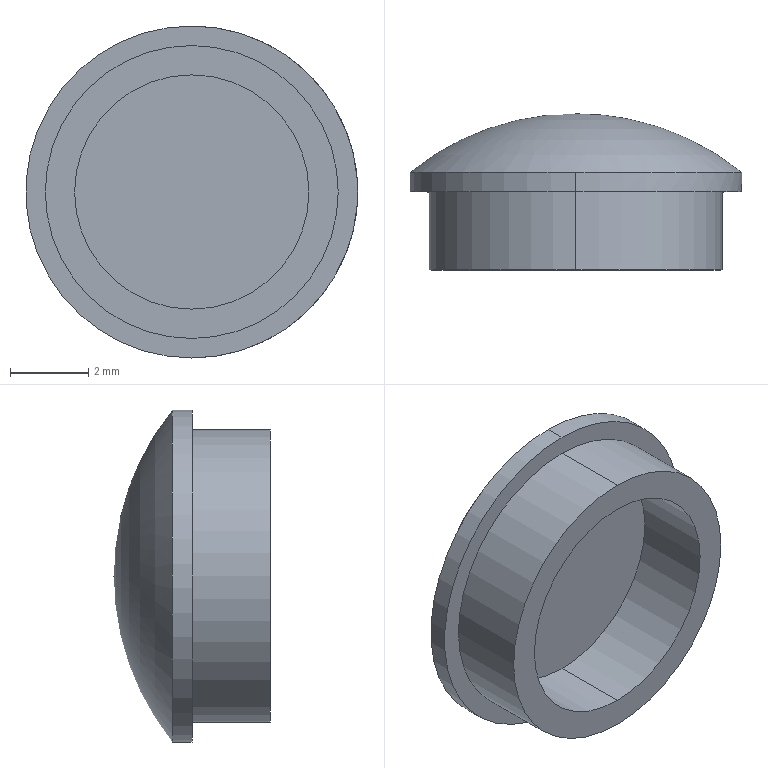Part | SolidWorks | features ICE 2, Dome 1, Extrusion 1, Scale 1 | 1 solid | 10 faces | box 8.5 x 4 x 8.5 mm | volume 104.507 mm3 | cylinder 6 | plane 3 | sphere 1 | commonest cylinder face diameters 6 x2 7.5 x2 8.5 x2
STEP:
#1=CARTESIAN_POINT('',(0.0000104,4.192,3.));
#2=VERTEX_POINT('',#1);
#3=CARTESIAN_POINT('',(0.0000104,4.192,-3.));
#4=VERTEX_POINT('',#3);
#5=CARTESIAN_POINT('',(0.0000104,4.192,0.0001016));
#6=DIRECTION('',(0.,-1.,0.));
#7=DIRECTION('',(0.,0.,-1.));
#8=AXIS2_PLACEMENT_3D('',#5,#6,#7);
#9=CIRCLE('',#8,3.);
#10=EDGE_CURVE('',#2,#4,#9,.T.);
#11=ORIENTED_EDGE('',*,*,#10,.F.);
#12=CARTESIAN_POINT('',(0.0000104,2.192,3.));
#13=VERTEX_POINT('',#12);
#14=CARTESIAN_POINT('',(0.0000104,4.192,3.));
#15=DIRECTION('',(0.,-1.,0.));
#16=VECTOR('',#15,1000.);
#17=LINE('',#14,#16);
#18=EDGE_CURVE('',#2,#13,#17,.T.);
#19=ORIENTED_EDGE('',*,*,#18,.T.);
#20=CARTESIAN_POINT('',(0.0000104,2.192,-3.));
#21=VERTEX_POINT('',#20);
#22=CARTESIAN_POINT('',(0.0000104,2.192,0.0001016));
#23=DIRECTION('',(0.,-1.,0.));
#24=DIRECTION('',(0.,0.,-1.));
#25=AXIS2_PLACEMENT_3D('',#22,#23,#24);
#26=CIRCLE('',#25,3.);
#27=EDGE_CURVE('',#13,#21,#26,.T.);
#28=ORIENTED_EDGE('',*,*,#27,.T.);
#29=CARTESIAN_POINT('',(0.0000104,4.192,-3.));
#30=DIRECTION('',(0.,-1.,0.));
#31=VECTOR('',#30,1000.);
#32=LINE('',#29,#31);
#33=EDGE_CURVE('',#4,#21,#32,.T.);
#34=ORIENTED_EDGE('',*,*,#33,.F.);
#35=EDGE_LOOP('',(#11,#19,#28,#34));
#36=FACE_OUTER_BOUND('',#35,.T.);
#37=CARTESIAN_POINT('',(0.0000104,4.192,0.0001016));
#38=DIRECTION('',(0.,-1.,0.));
#39=DIRECTION('',(0.,0.,-1.));
#40=AXIS2_PLACEMENT_3D('',#37,#38,#39);
#41=CYLINDRICAL_SURFACE('',#40,3.);
#42=ADVANCED_FACE('',(#36),#41,.F.);
#43=CARTESIAN_POINT('',(0.0000104,4.692,4.25));
#44=VERTEX_POINT('',#43);
#45=CARTESIAN_POINT('',(0.0000104,4.692,-4.25));
#46=VERTEX_POINT('',#45);
#47=CARTESIAN_POINT('',(0.0000104,4.692,0.0001016));
#48=DIRECTION('',(0.,1.,0.));
#49=DIRECTION('',(0.,0.,1.));
#50=AXIS2_PLACEMENT_3D('',#47,#48,#49);
#51=CIRCLE('',#50,4.25);
#52=EDGE_CURVE('',#44,#46,#51,.T.);
#53=ORIENTED_EDGE('',*,*,#52,.F.);
#54=CARTESIAN_POINT('',(0.0000104,4.192,4.25));
#55=VERTEX_POINT('',#54);
#56=CARTESIAN_POINT('',(0.0000104,4.692,4.25));
#57=DIRECTION('',(0.,-1.,0.));
#58=VECTOR('',#57,1000.);
#59=LINE('',#56,#58);
#60=EDGE_CURVE('',#44,#55,#59,.T.);
#61=ORIENTED_EDGE('',*,*,#60,.T.);
#62=CARTESIAN_POINT('',(0.0000104,4.192,-4.25));
#63=VERTEX_POINT('',#62);
#64=CARTESIAN_POINT('',(0.0000104,4.192,0.0001016));
#65=DIRECTION('',(0.,1.,0.));
#66=DIRECTION('',(0.,0.,1.));
#67=AXIS2_PLACEMENT_3D('',#64,#65,#66);
#68=CIRCLE('',#67,4.25);
#69=EDGE_CURVE('',#55,#63,#68,.T.);
#70=ORIENTED_EDGE('',*,*,#69,.T.);
#71=CARTESIAN_POINT('',(0.0000104,4.692,-4.25));
#72=DIRECTION('',(0.,-1.,0.));
#73=VECTOR('',#72,1000.);
#74=LINE('',#71,#73);
#75=EDGE_CURVE('',#46,#63,#74,.T.);
#76=ORIENTED_EDGE('',*,*,#75,.F.);
#77=EDGE_LOOP('',(#53,#61,#70,#76));
#78=FACE_OUTER_BOUND('',#77,.T.);
#79=CARTESIAN_POINT('',(0.0000104,4.692,0.0001016));
#80=DIRECTION('',(0.,-1.,0.));
#81=DIRECTION('',(0.,0.,-1.));
#82=AXIS2_PLACEMENT_3D('',#79,#80,#81);
#83=CYLINDRICAL_SURFACE('',#82,4.25);
#84=ADVANCED_FACE('',(#78),#83,.T.);
#85=CARTESIAN_POINT('',(0.0000104,4.192,3.75));
#86=VERTEX_POINT('',#85);
#87=CARTESIAN_POINT('',(0.0000104,4.192,-3.75));
#88=VERTEX_POINT('',#87);
#89=CARTESIAN_POINT('',(0.0000104,4.192,0.0001016));
#90=DIRECTION('',(0.,1.,0.));
#91=DIRECTION('',(0.,0.,1.));
#92=AXIS2_PLACEMENT_3D('',#89,#90,#91);
#93=CIRCLE('',#92,3.75);
#94=EDGE_CURVE('',#86,#88,#93,.T.);
#95=ORIENTED_EDGE('',*,*,#94,.F.);
#96=CARTESIAN_POINT('',(0.0000104,2.192,3.75));
#97=VERTEX_POINT('',#96);
#98=CARTESIAN_POINT('',(0.0000104,4.192,3.75));
#99=DIRECTION('',(0.,-1.,0.));
#100=VECTOR('',#99,1000.);
#101=LINE('',#98,#100);
#102=EDGE_CURVE('',#86,#97,#101,.T.);
#103=ORIENTED_EDGE('',*,*,#102,.T.);
#104=CARTESIAN_POINT('',(0.0000104,2.192,-3.75));
#105=VERTEX_POINT('',#104);
#106=CARTESIAN_POINT('',(0.0000104,2.192,0.0001016));
#107=DIRECTION('',(0.,1.,0.));
#108=DIRECTION('',(0.,0.,1.));
#109=AXIS2_PLACEMENT_3D('',#106,#107,#108);
#110=CIRCLE('',#109,3.75);
#111=EDGE_CURVE('',#97,#105,#110,.T.);
#112=ORIENTED_EDGE('',*,*,#111,.T.);
#113=CARTESIAN_POINT('',(0.0000104,4.192,-3.75));
#114=DIRECTION('',(0.,-1.,0.));
#115=VECTOR('',#114,1000.);
#116=LINE('',#113,#115);
#117=EDGE_CURVE('',#88,#105,#116,.T.);
#118=ORIENTED_EDGE('',*,*,#117,.F.);
#119=EDGE_LOOP('',(#95,#103,#112,#118));
#120=FACE_OUTER_BOUND('',#119,.T.);
#121=CARTESIAN_POINT('',(0.0000104,4.192,0.0001016));
#122=DIRECTION('',(0.,-1.,0.));
#123=DIRECTION('',(0.,0.,-1.));
#124=AXIS2_PLACEMENT_3D('',#121,#122,#123);
#125=CYLINDRICAL_SURFACE('',#124,3.75);
#126=ADVANCED_FACE('',(#120),#125,.T.);
#127=ORIENTED_EDGE('',*,*,#102,.F.);
#128=CARTESIAN_POINT('',(0.0000104,4.192,0.0001016));
#129=DIRECTION('',(0.,1.,0.));
#130=DIRECTION('',(0.,0.,1.));
#131=AXIS2_PLACEMENT_3D('',#128,#129,#130);
#132=CIRCLE('',#131,3.75);
#133=EDGE_CURVE('',#88,#86,#132,.T.);
#134=ORIENTED_EDGE('',*,*,#133,.F.);
#135=ORIENTED_EDGE('',*,*,#117,.T.);
#136=CARTESIAN_POINT('',(0.0000104,2.192,0.0001016));
#137=DIRECTION('',(0.,1.,0.));
#138=DIRECTION('',(0.,0.,1.));
#139=AXIS2_PLACEMENT_3D('',#136,#137,#138);
#140=CIRCLE('',#139,3.75);
#141=EDGE_CURVE('',#105,#97,#140,.T.);
#142=ORIENTED_EDGE('',*,*,#141,.T.);
#143=EDGE_LOOP('',(#127,#134,#135,#142));
#144=FACE_OUTER_BOUND('',#143,.T.);
#145=CARTESIAN_POINT('',(0.0000104,4.192,0.0001016));
#146=DIRECTION('',(0.,-1.,0.));
#147=DIRECTION('',(0.,0.,-1.));
#148=AXIS2_PLACEMENT_3D('',#145,#146,#147);
#149=CYLINDRICAL_SURFACE('',#148,3.75);
#150=ADVANCED_FACE('',(#144),#149,.T.);
#151=CARTESIAN_POINT('',(0.0000104,2.192,0.0001016));
#152=DIRECTION('',(0.,-1.,0.));
#153=DIRECTION('',(0.,0.,-1.));
#154=AXIS2_PLACEMENT_3D('',#151,#152,#153);
#155=CIRCLE('',#154,3.);
#156=EDGE_CURVE('',#21,#13,#155,.T.);
#157=ORIENTED_EDGE('',*,*,#156,.F.);
#158=ORIENTED_EDGE('',*,*,#27,.F.);
#159=EDGE_LOOP('',(#157,#158));
#160=FACE_BOUND('',#159,.T.);
#161=ORIENTED_EDGE('',*,*,#141,.F.);
#162=ORIENTED_EDGE('',*,*,#111,.F.);
#163=EDGE_LOOP('',(#161,#162));
#164=FACE_OUTER_BOUND('',#163,.T.);
#165=CARTESIAN_POINT('',(0.0000104,2.192,0.0001016));
#166=DIRECTION('',(0.,1.,0.));
#167=DIRECTION('',(0.,0.,1.));
#168=AXIS2_PLACEMENT_3D('',#165,#166,#167);
#169=PLANE('',#168);
#170=ADVANCED_FACE('',(#160,#164),#169,.F.);
#171=ORIENTED_EDGE('',*,*,#60,.F.);
#172=CARTESIAN_POINT('',(0.0000104,4.692,0.0001016));
#173=DIRECTION('',(0.,1.,0.));
#174=DIRECTION('',(0.,0.,1.));
#175=AXIS2_PLACEMENT_3D('',#172,#173,#174);
#176=CIRCLE('',#175,4.25);
#177=EDGE_CURVE('',#46,#44,#176,.T.);
#178=ORIENTED_EDGE('',*,*,#177,.F.);
#179=ORIENTED_EDGE('',*,*,#75,.T.);
#180=CARTESIAN_POINT('',(0.0000104,4.192,0.0001016));
#181=DIRECTION('',(0.,1.,0.));
#182=DIRECTION('',(0.,0.,1.));
#183=AXIS2_PLACEMENT_3D('',#180,#181,#182);
#184=CIRCLE('',#183,4.25);
#185=EDGE_CURVE('',#63,#55,#184,.T.);
#186=ORIENTED_EDGE('',*,*,#185,.T.);
#187=EDGE_LOOP('',(#171,#178,#179,#186));
#188=FACE_OUTER_BOUND('',#187,.T.);
#189=CARTESIAN_POINT('',(0.0000104,4.692,0.0001016));
#190=DIRECTION('',(0.,-1.,0.));
#191=DIRECTION('',(0.,0.,-1.));
#192=AXIS2_PLACEMENT_3D('',#189,#190,#191);
#193=CYLINDRICAL_SURFACE('',#192,4.25);
#194=ADVANCED_FACE('',(#188),#193,.T.);
#195=ORIENTED_EDGE('',*,*,#177,.T.);
#196=ORIENTED_EDGE('',*,*,#52,.T.);
#197=EDGE_LOOP('',(#195,#196));
#198=FACE_OUTER_BOUND('',#197,.T.);
#199=CARTESIAN_POINT('',(0.0000104,-0.5789,0.0001016));
#200=DIRECTION('',(0.,1.,0.));
#201=DIRECTION('',(1.,0.,0.));
#202=AXIS2_PLACEMENT_3D('',#199,#200,#201);
#203=SPHERICAL_SURFACE('',#202,6.771);
#204=ADVANCED_FACE('',(#198),#203,.T.);
#205=ORIENTED_EDGE('',*,*,#133,.T.);
#206=ORIENTED_EDGE('',*,*,#94,.T.);
#207=EDGE_LOOP('',(#205,#206));
#208=FACE_BOUND('',#207,.T.);
#209=ORIENTED_EDGE('',*,*,#185,.F.);
#210=ORIENTED_EDGE('',*,*,#69,.F.);
#211=EDGE_LOOP('',(#209,#210));
#212=FACE_OUTER_BOUND('',#211,.T.);
#213=CARTESIAN_POINT('',(0.0000104,4.192,0.0001016));
#214=DIRECTION('',(0.,1.,0.));
#215=DIRECTION('',(0.,0.,1.));
#216=AXIS2_PLACEMENT_3D('',#213,#214,#215);
#217=PLANE('',#216);
#218=ADVANCED_FACE('',(#208,#212),#217,.F.);
#219=ORIENTED_EDGE('',*,*,#18,.F.);
#220=CARTESIAN_POINT('',(0.0000104,4.192,0.0001016));
#221=DIRECTION('',(0.,-1.,0.));
#222=DIRECTION('',(0.,0.,-1.));
#223=AXIS2_PLACEMENT_3D('',#220,#221,#222);
#224=CIRCLE('',#223,3.);
#225=EDGE_CURVE('',#4,#2,#224,.T.);
#226=ORIENTED_EDGE('',*,*,#225,.F.);
#227=ORIENTED_EDGE('',*,*,#33,.T.);
#228=ORIENTED_EDGE('',*,*,#156,.T.);
#229=EDGE_LOOP('',(#219,#226,#227,#228));
#230=FACE_OUTER_BOUND('',#229,.T.);
#231=CARTESIAN_POINT('',(0.0000104,4.192,0.0001016));
#232=DIRECTION('',(0.,-1.,0.));
#233=DIRECTION('',(0.,0.,-1.));
#234=AXIS2_PLACEMENT_3D('',#231,#232,#233);
#235=CYLINDRICAL_SURFACE('',#234,3.);
#236=ADVANCED_FACE('',(#230),#235,.F.);
#237=ORIENTED_EDGE('',*,*,#225,.T.);
#238=ORIENTED_EDGE('',*,*,#10,.T.);
#239=EDGE_LOOP('',(#237,#238));
#240=FACE_OUTER_BOUND('',#239,.T.);
#241=CARTESIAN_POINT('',(0.0000104,4.192,0.0001016));
#242=DIRECTION('',(0.,-1.,0.));
#243=DIRECTION('',(0.,0.,-1.));
#244=AXIS2_PLACEMENT_3D('',#241,#242,#243);
#245=PLANE('',#244);
#246=ADVANCED_FACE('',(#240),#245,.T.);
#247=CLOSED_SHELL('',(#42,#84,#126,#150,#170,#194,#204,#218,#236,#246));
#248=MANIFOLD_SOLID_BREP('',#247);
#249=CARTESIAN_POINT('',(0.,0.,0.));
#250=DIRECTION('',(0.,0.,1.));
#251=DIRECTION('',(1.,0.,0.));
#252=AXIS2_PLACEMENT_3D('',#249,#250,#251);
#253=(LENGTH_UNIT()NAMED_UNIT(*)SI_UNIT(.MILLI.,.METRE.));
#254=UNCERTAINTY_MEASURE_WITH_UNIT(LENGTH_MEASURE(0.00001),#253,'','');
#255=(NAMED_UNIT(*)PLANE_ANGLE_UNIT()SI_UNIT($,.RADIAN.));
#256=(NAMED_UNIT(*)SI_UNIT($,.STERADIAN.)SOLID_ANGLE_UNIT());
#257=(GEOMETRIC_REPRESENTATION_CONTEXT(3)GLOBAL_UNCERTAINTY_ASSIGNED_CONTEXT((#254))GLOBAL_UNIT_ASSIGNED_CONTEXT((#253,#255,#256))REPRESENTATION_CONTEXT('',''));
#258=ADVANCED_BREP_SHAPE_REPRESENTATION('',(#248,#252),#257);